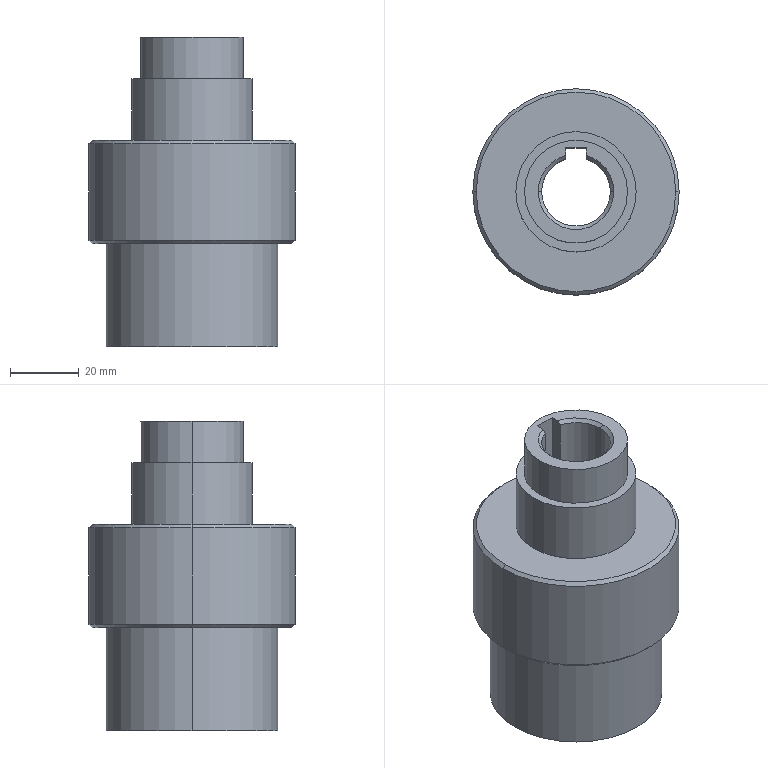Part | SolidWorks | features ICE 8, HoleWzd 2, Chamfer 1, Extrusion 1 | 1 solid | 31 faces | box 60 x 60 x 90 mm | volume 128146 mm3 | cylinder 13 | cone 9 | plane 9 | commonest cylinder face diameters 30 x4 20 x3 35 x2 50 x2 60 x2
STEP:
#1=CARTESIAN_POINT('',(15.,0.,1.));
#2=VERTEX_POINT('',#1);
#3=CARTESIAN_POINT('',(-15.,0.,1.));
#4=VERTEX_POINT('',#3);
#5=CARTESIAN_POINT('',(0.,0.,1.));
#6=DIRECTION('',(0.,0.,-1.));
#7=DIRECTION('',(1.,0.,0.));
#8=AXIS2_PLACEMENT_3D('',#5,#6,#7);
#9=CIRCLE('',#8,15.);
#10=EDGE_CURVE('',#2,#4,#9,.T.);
#11=ORIENTED_EDGE('',*,*,#10,.F.);
#12=CARTESIAN_POINT('',(16.,0.,0.));
#13=VERTEX_POINT('',#12);
#14=CARTESIAN_POINT('',(15.,0.,1.));
#15=DIRECTION('',(0.7071,0.,-0.7071));
#16=VECTOR('',#15,1000.);
#17=LINE('',#14,#16);
#18=EDGE_CURVE('',#2,#13,#17,.T.);
#19=ORIENTED_EDGE('',*,*,#18,.T.);
#20=CARTESIAN_POINT('',(-16.,0.,0.));
#21=VERTEX_POINT('',#20);
#22=CARTESIAN_POINT('',(0.,0.,0.));
#23=DIRECTION('',(0.,0.,1.));
#24=DIRECTION('',(1.,0.,0.));
#25=AXIS2_PLACEMENT_3D('',#22,#23,#24);
#26=CIRCLE('',#25,16.);
#27=EDGE_CURVE('',#21,#13,#26,.T.);
#28=ORIENTED_EDGE('',*,*,#27,.F.);
#29=CARTESIAN_POINT('',(-15.,0.,1.));
#30=DIRECTION('',(-0.7071,0.,-0.7071));
#31=VECTOR('',#30,1000.);
#32=LINE('',#29,#31);
#33=EDGE_CURVE('',#4,#21,#32,.T.);
#34=ORIENTED_EDGE('',*,*,#33,.F.);
#35=EDGE_LOOP('',(#11,#19,#28,#34));
#36=FACE_OUTER_BOUND('',#35,.T.);
#37=CARTESIAN_POINT('',(0.,0.,1.));
#38=DIRECTION('',(0.,0.,-1.));
#39=DIRECTION('',(-1.,0.,0.));
#40=AXIS2_PLACEMENT_3D('',#37,#38,#39);
#41=CONICAL_SURFACE('',#40,15.,0.7854);
#42=ADVANCED_FACE('',(#36),#41,.F.);
#43=CARTESIAN_POINT('',(-10.,0.,89.));
#44=VERTEX_POINT('',#43);
#45=CARTESIAN_POINT('',(10.,0.,89.));
#46=VERTEX_POINT('',#45);
#47=CARTESIAN_POINT('',(0.,0.,89.));
#48=DIRECTION('',(0.,0.,1.));
#49=DIRECTION('',(1.,0.,0.));
#50=AXIS2_PLACEMENT_3D('',#47,#48,#49);
#51=CIRCLE('',#50,10.);
#52=EDGE_CURVE('',#44,#46,#51,.T.);
#53=ORIENTED_EDGE('',*,*,#52,.F.);
#54=CARTESIAN_POINT('',(-11.,0.,90.));
#55=VERTEX_POINT('',#54);
#56=CARTESIAN_POINT('',(-10.,0.,89.));
#57=DIRECTION('',(-0.7071,0.,0.7071));
#58=VECTOR('',#57,1000.);
#59=LINE('',#56,#58);
#60=EDGE_CURVE('',#44,#55,#59,.T.);
#61=ORIENTED_EDGE('',*,*,#60,.T.);
#62=CARTESIAN_POINT('',(11.,0.,90.));
#63=VERTEX_POINT('',#62);
#64=CARTESIAN_POINT('',(0.,0.,90.));
#65=DIRECTION('',(0.,0.,-1.));
#66=DIRECTION('',(1.,0.,0.));
#67=AXIS2_PLACEMENT_3D('',#64,#65,#66);
#68=CIRCLE('',#67,11.);
#69=EDGE_CURVE('',#63,#55,#68,.T.);
#70=ORIENTED_EDGE('',*,*,#69,.F.);
#71=CARTESIAN_POINT('',(10.,0.,89.));
#72=DIRECTION('',(0.7071,0.,0.7071));
#73=VECTOR('',#72,1000.);
#74=LINE('',#71,#73);
#75=EDGE_CURVE('',#46,#63,#74,.T.);
#76=ORIENTED_EDGE('',*,*,#75,.F.);
#77=EDGE_LOOP('',(#53,#61,#70,#76));
#78=FACE_OUTER_BOUND('',#77,.T.);
#79=CARTESIAN_POINT('',(0.,0.,89.));
#80=DIRECTION('',(0.,0.,1.));
#81=DIRECTION('',(1.,0.,0.));
#82=AXIS2_PLACEMENT_3D('',#79,#80,#81);
#83=CONICAL_SURFACE('',#82,10.,0.7854);
#84=ADVANCED_FACE('',(#78),#83,.F.);
#85=CARTESIAN_POINT('',(3.,9.539,89.));
#86=VERTEX_POINT('',#85);
#87=CARTESIAN_POINT('',(0.,0.,89.));
#88=DIRECTION('',(0.,0.,1.));
#89=DIRECTION('',(1.,0.,0.));
#90=AXIS2_PLACEMENT_3D('',#87,#88,#89);
#91=CIRCLE('',#90,10.);
#92=EDGE_CURVE('',#46,#86,#91,.T.);
#93=ORIENTED_EDGE('',*,*,#92,.F.);
#94=ORIENTED_EDGE('',*,*,#75,.T.);
#95=CARTESIAN_POINT('',(3.,10.583,90.));
#96=VERTEX_POINT('',#95);
#97=CARTESIAN_POINT('',(0.,0.,90.));
#98=DIRECTION('',(0.,0.,-1.));
#99=DIRECTION('',(1.,0.,0.));
#100=AXIS2_PLACEMENT_3D('',#97,#98,#99);
#101=CIRCLE('',#100,11.);
#102=EDGE_CURVE('',#96,#63,#101,.T.);
#103=ORIENTED_EDGE('',*,*,#102,.F.);
#104=CARTESIAN_POINT('',(3.,9.539,89.));
#105=CARTESIAN_POINT('',(3.,9.888,89.333));
#106=CARTESIAN_POINT('',(3.,10.236,89.666));
#107=CARTESIAN_POINT('',(3.,10.583,90.));
#108=B_SPLINE_CURVE_WITH_KNOTS('',3,(#104,#105,#106,#107),.UNSPECIFIED.,.F.,.F.,(4,4),(0.,0.001445),.UNSPECIFIED.);
#109=EDGE_CURVE('',#86,#96,#108,.T.);
#110=ORIENTED_EDGE('',*,*,#109,.F.);
#111=EDGE_LOOP('',(#93,#94,#103,#110));
#112=FACE_OUTER_BOUND('',#111,.T.);
#113=CARTESIAN_POINT('',(0.,0.,89.));
#114=DIRECTION('',(0.,0.,1.));
#115=DIRECTION('',(1.,0.,0.));
#116=AXIS2_PLACEMENT_3D('',#113,#114,#115);
#117=CONICAL_SURFACE('',#116,10.,0.7854);
#118=ADVANCED_FACE('',(#112),#117,.F.);
#119=CARTESIAN_POINT('',(-29.,0.,30.));
#120=VERTEX_POINT('',#119);
#121=CARTESIAN_POINT('',(29.,0.,30.));
#122=VERTEX_POINT('',#121);
#123=CARTESIAN_POINT('',(0.,0.,30.));
#124=DIRECTION('',(0.,0.,-1.));
#125=DIRECTION('',(1.,0.,0.));
#126=AXIS2_PLACEMENT_3D('',#123,#124,#125);
#127=CIRCLE('',#126,29.);
#128=EDGE_CURVE('',#120,#122,#127,.T.);
#129=ORIENTED_EDGE('',*,*,#128,.F.);
#130=CARTESIAN_POINT('',(-30.,0.,31.));
#131=VERTEX_POINT('',#130);
#132=CARTESIAN_POINT('',(-30.,0.,31.));
#133=DIRECTION('',(-0.7071,0.,0.7071));
#134=VECTOR('',#133,1000.);
#135=LINE('',#132,#134);
#136=EDGE_CURVE('',#120,#131,#135,.T.);
#137=ORIENTED_EDGE('',*,*,#136,.T.);
#138=CARTESIAN_POINT('',(30.,0.,31.));
#139=VERTEX_POINT('',#138);
#140=CARTESIAN_POINT('',(0.,0.,31.));
#141=DIRECTION('',(0.,0.,1.));
#142=DIRECTION('',(1.,0.,0.));
#143=AXIS2_PLACEMENT_3D('',#140,#141,#142);
#144=CIRCLE('',#143,30.);
#145=EDGE_CURVE('',#139,#131,#144,.T.);
#146=ORIENTED_EDGE('',*,*,#145,.F.);
#147=CARTESIAN_POINT('',(30.,0.,31.));
#148=DIRECTION('',(0.7071,0.,0.7071));
#149=VECTOR('',#148,1000.);
#150=LINE('',#147,#149);
#151=EDGE_CURVE('',#122,#139,#150,.T.);
#152=ORIENTED_EDGE('',*,*,#151,.F.);
#153=EDGE_LOOP('',(#129,#137,#146,#152));
#154=FACE_OUTER_BOUND('',#153,.T.);
#155=CARTESIAN_POINT('',(0.,0.,31.));
#156=DIRECTION('',(0.,0.,1.));
#157=DIRECTION('',(1.,0.,0.));
#158=AXIS2_PLACEMENT_3D('',#155,#156,#157);
#159=CONICAL_SURFACE('',#158,30.,0.7854);
#160=ADVANCED_FACE('',(#154),#159,.T.);
#161=CARTESIAN_POINT('',(29.,0.,60.));
#162=VERTEX_POINT('',#161);
#163=CARTESIAN_POINT('',(-29.,0.,60.));
#164=VERTEX_POINT('',#163);
#165=CARTESIAN_POINT('',(0.,0.,60.));
#166=DIRECTION('',(0.,0.,1.));
#167=DIRECTION('',(1.,0.,0.));
#168=AXIS2_PLACEMENT_3D('',#165,#166,#167);
#169=CIRCLE('',#168,29.);
#170=EDGE_CURVE('',#162,#164,#169,.T.);
#171=ORIENTED_EDGE('',*,*,#170,.F.);
#172=CARTESIAN_POINT('',(30.,0.,59.));
#173=VERTEX_POINT('',#172);
#174=CARTESIAN_POINT('',(29.,0.,60.));
#175=DIRECTION('',(0.7071,0.,-0.7071));
#176=VECTOR('',#175,1000.);
#177=LINE('',#174,#176);
#178=EDGE_CURVE('',#162,#173,#177,.T.);
#179=ORIENTED_EDGE('',*,*,#178,.T.);
#180=CARTESIAN_POINT('',(-30.,0.,59.));
#181=VERTEX_POINT('',#180);
#182=CARTESIAN_POINT('',(0.,0.,59.));
#183=DIRECTION('',(0.,0.,-1.));
#184=DIRECTION('',(1.,0.,0.));
#185=AXIS2_PLACEMENT_3D('',#182,#183,#184);
#186=CIRCLE('',#185,30.);
#187=EDGE_CURVE('',#181,#173,#186,.T.);
#188=ORIENTED_EDGE('',*,*,#187,.F.);
#189=CARTESIAN_POINT('',(-29.,0.,60.));
#190=DIRECTION('',(-0.7071,0.,-0.7071));
#191=VECTOR('',#190,1000.);
#192=LINE('',#189,#191);
#193=EDGE_CURVE('',#164,#181,#192,.T.);
#194=ORIENTED_EDGE('',*,*,#193,.F.);
#195=EDGE_LOOP('',(#171,#179,#188,#194));
#196=FACE_OUTER_BOUND('',#195,.T.);
#197=CARTESIAN_POINT('',(0.,0.,60.));
#198=DIRECTION('',(0.,0.,-1.));
#199=DIRECTION('',(-1.,0.,0.));
#200=AXIS2_PLACEMENT_3D('',#197,#198,#199);
#201=CONICAL_SURFACE('',#200,29.,0.7854);
#202=ADVANCED_FACE('',(#196),#201,.T.);
#203=CARTESIAN_POINT('',(15.,0.,78.));
#204=VERTEX_POINT('',#203);
#205=CARTESIAN_POINT('',(-15.,0.,78.));
#206=VERTEX_POINT('',#205);
#207=CARTESIAN_POINT('',(0.,0.,78.));
#208=DIRECTION('',(0.,0.,1.));
#209=DIRECTION('',(1.,0.,0.));
#210=AXIS2_PLACEMENT_3D('',#207,#208,#209);
#211=CIRCLE('',#210,15.);
#212=EDGE_CURVE('',#204,#206,#211,.T.);
#213=ORIENTED_EDGE('',*,*,#212,.T.);
#214=CARTESIAN_POINT('',(-15.,0.,90.));
#215=VERTEX_POINT('',#214);
#216=CARTESIAN_POINT('',(-15.,0.,78.));
#217=DIRECTION('',(0.,0.,1.));
#218=VECTOR('',#217,1000.);
#219=LINE('',#216,#218);
#220=EDGE_CURVE('',#206,#215,#219,.T.);
#221=ORIENTED_EDGE('',*,*,#220,.T.);
#222=CARTESIAN_POINT('',(15.,0.,90.));
#223=VERTEX_POINT('',#222);
#224=CARTESIAN_POINT('',(0.,0.,90.));
#225=DIRECTION('',(0.,0.,1.));
#226=DIRECTION('',(1.,0.,0.));
#227=AXIS2_PLACEMENT_3D('',#224,#225,#226);
#228=CIRCLE('',#227,15.);
#229=EDGE_CURVE('',#223,#215,#228,.T.);
#230=ORIENTED_EDGE('',*,*,#229,.F.);
#231=CARTESIAN_POINT('',(15.,0.,78.));
#232=DIRECTION('',(0.,0.,1.));
#233=VECTOR('',#232,1000.);
#234=LINE('',#231,#233);
#235=EDGE_CURVE('',#204,#223,#234,.T.);
#236=ORIENTED_EDGE('',*,*,#235,.F.);
#237=EDGE_LOOP('',(#213,#221,#230,#236));
#238=FACE_OUTER_BOUND('',#237,.T.);
#239=CARTESIAN_POINT('',(0.,0.,78.));
#240=DIRECTION('',(0.,0.,1.));
#241=DIRECTION('',(1.,0.,0.));
#242=AXIS2_PLACEMENT_3D('',#239,#240,#241);
#243=CYLINDRICAL_SURFACE('',#242,15.);
#244=ADVANCED_FACE('',(#238),#243,.T.);
#245=CARTESIAN_POINT('',(15.,0.,30.));
#246=VERTEX_POINT('',#245);
#247=CARTESIAN_POINT('',(-15.,0.,30.));
#248=VERTEX_POINT('',#247);
#249=CARTESIAN_POINT('',(0.,0.,30.));
#250=DIRECTION('',(0.,0.,-1.));
#251=DIRECTION('',(-1.,0.,0.));
#252=AXIS2_PLACEMENT_3D('',#249,#250,#251);
#253=CIRCLE('',#252,15.);
#254=EDGE_CURVE('',#246,#248,#253,.T.);
#255=ORIENTED_EDGE('',*,*,#254,.F.);
#256=CARTESIAN_POINT('',(15.,0.,30.));
#257=DIRECTION('',(0.,0.,-1.));
#258=VECTOR('',#257,1000.);
#259=LINE('',#256,#258);
#260=EDGE_CURVE('',#246,#2,#259,.T.);
#261=ORIENTED_EDGE('',*,*,#260,.T.);
#262=ORIENTED_EDGE('',*,*,#10,.T.);
#263=CARTESIAN_POINT('',(-15.,0.,30.));
#264=DIRECTION('',(0.,0.,-1.));
#265=VECTOR('',#264,1000.);
#266=LINE('',#263,#265);
#267=EDGE_CURVE('',#248,#4,#266,.T.);
#268=ORIENTED_EDGE('',*,*,#267,.F.);
#269=EDGE_LOOP('',(#255,#261,#262,#268));
#270=FACE_OUTER_BOUND('',#269,.T.);
#271=CARTESIAN_POINT('',(0.,0.,30.));
#272=DIRECTION('',(0.,0.,-1.));
#273=DIRECTION('',(-1.,0.,0.));
#274=AXIS2_PLACEMENT_3D('',#271,#272,#273);
#275=CYLINDRICAL_SURFACE('',#274,15.);
#276=ADVANCED_FACE('',(#270),#275,.F.);
#277=CARTESIAN_POINT('',(25.,0.,30.));
#278=VERTEX_POINT('',#277);
#279=CARTESIAN_POINT('',(-25.,0.,30.));
#280=VERTEX_POINT('',#279);
#281=CARTESIAN_POINT('',(0.,0.,30.));
#282=DIRECTION('',(0.,0.,1.));
#283=DIRECTION('',(1.,0.,0.));
#284=AXIS2_PLACEMENT_3D('',#281,#282,#283);
#285=CIRCLE('',#284,25.);
#286=EDGE_CURVE('',#278,#280,#285,.T.);
#287=ORIENTED_EDGE('',*,*,#286,.F.);
#288=CARTESIAN_POINT('',(25.,0.,0.));
#289=VERTEX_POINT('',#288);
#290=CARTESIAN_POINT('',(25.,0.,30.));
#291=DIRECTION('',(0.,0.,-1.));
#292=VECTOR('',#291,1000.);
#293=LINE('',#290,#292);
#294=EDGE_CURVE('',#278,#289,#293,.T.);
#295=ORIENTED_EDGE('',*,*,#294,.T.);
#296=CARTESIAN_POINT('',(-25.,0.,0.));
#297=VERTEX_POINT('',#296);
#298=CARTESIAN_POINT('',(0.,0.,0.));
#299=DIRECTION('',(0.,0.,1.));
#300=DIRECTION('',(1.,0.,0.));
#301=AXIS2_PLACEMENT_3D('',#298,#299,#300);
#302=CIRCLE('',#301,25.);
#303=EDGE_CURVE('',#289,#297,#302,.T.);
#304=ORIENTED_EDGE('',*,*,#303,.T.);
#305=CARTESIAN_POINT('',(-25.,0.,30.));
#306=DIRECTION('',(0.,0.,-1.));
#307=VECTOR('',#306,1000.);
#308=LINE('',#305,#307);
#309=EDGE_CURVE('',#280,#297,#308,.T.);
#310=ORIENTED_EDGE('',*,*,#309,.F.);
#311=EDGE_LOOP('',(#287,#295,#304,#310));
#312=FACE_OUTER_BOUND('',#311,.T.);
#313=CARTESIAN_POINT('',(0.,0.,30.));
#314=DIRECTION('',(0.,0.,-1.));
#315=DIRECTION('',(-1.,0.,0.));
#316=AXIS2_PLACEMENT_3D('',#313,#314,#315);
#317=CYLINDRICAL_SURFACE('',#316,25.);
#318=ADVANCED_FACE('',(#312),#317,.T.);
#319=ORIENTED_EDGE('',*,*,#52,.T.);
#320=CARTESIAN_POINT('',(10.,0.,30.));
#321=VERTEX_POINT('',#320);
#322=CARTESIAN_POINT('',(10.,0.,70.));
#323=DIRECTION('',(0.,0.,-1.));
#324=VECTOR('',#323,1000.);
#325=LINE('',#322,#324);
#326=EDGE_CURVE('',#46,#321,#325,.T.);
#327=ORIENTED_EDGE('',*,*,#326,.T.);
#328=CARTESIAN_POINT('',(-10.,0.,30.));
#329=VERTEX_POINT('',#328);
#330=CARTESIAN_POINT('',(0.,0.,30.));
#331=DIRECTION('',(0.,0.,1.));
#332=DIRECTION('',(-1.,0.,0.));
#333=AXIS2_PLACEMENT_3D('',#330,#331,#332);
#334=CIRCLE('',#333,10.);
#335=EDGE_CURVE('',#329,#321,#334,.T.);
#336=ORIENTED_EDGE('',*,*,#335,.F.);
#337=CARTESIAN_POINT('',(-10.,0.,70.));
#338=DIRECTION('',(0.,0.,-1.));
#339=VECTOR('',#338,1000.);
#340=LINE('',#337,#339);
#341=EDGE_CURVE('',#44,#329,#340,.T.);
#342=ORIENTED_EDGE('',*,*,#341,.F.);
#343=EDGE_LOOP('',(#319,#327,#336,#342));
#344=FACE_OUTER_BOUND('',#343,.T.);
#345=CARTESIAN_POINT('',(0.,0.,70.));
#346=DIRECTION('',(0.,0.,-1.));
#347=DIRECTION('',(-1.,0.,0.));
#348=AXIS2_PLACEMENT_3D('',#345,#346,#347);
#349=CYLINDRICAL_SURFACE('',#348,10.);
#350=ADVANCED_FACE('',(#344),#349,.F.);
#351=CARTESIAN_POINT('',(-3.,9.539,89.));
#352=VERTEX_POINT('',#351);
#353=CARTESIAN_POINT('',(0.,0.,89.));
#354=DIRECTION('',(0.,0.,1.));
#355=DIRECTION('',(1.,0.,0.));
#356=AXIS2_PLACEMENT_3D('',#353,#354,#355);
#357=CIRCLE('',#356,10.);
#358=EDGE_CURVE('',#352,#44,#357,.T.);
#359=ORIENTED_EDGE('',*,*,#358,.T.);
#360=ORIENTED_EDGE('',*,*,#341,.T.);
#361=CARTESIAN_POINT('',(-3.,9.539,30.));
#362=VERTEX_POINT('',#361);
#363=CARTESIAN_POINT('',(0.,0.,30.));
#364=DIRECTION('',(0.,0.,1.));
#365=DIRECTION('',(-1.,0.,0.));
#366=AXIS2_PLACEMENT_3D('',#363,#364,#365);
#367=CIRCLE('',#366,10.);
#368=EDGE_CURVE('',#362,#329,#367,.T.);
#369=ORIENTED_EDGE('',*,*,#368,.F.);
#370=CARTESIAN_POINT('',(-3.,9.539,0.));
#371=DIRECTION('',(0.,0.,1.));
#372=VECTOR('',#371,1000.);
#373=LINE('',#370,#372);
#374=EDGE_CURVE('',#362,#352,#373,.T.);
#375=ORIENTED_EDGE('',*,*,#374,.T.);
#376=EDGE_LOOP('',(#359,#360,#369,#375));
#377=FACE_OUTER_BOUND('',#376,.T.);
#378=CARTESIAN_POINT('',(0.,0.,70.));
#379=DIRECTION('',(0.,0.,-1.));
#380=DIRECTION('',(-1.,0.,0.));
#381=AXIS2_PLACEMENT_3D('',#378,#379,#380);
#382=CYLINDRICAL_SURFACE('',#381,10.);
#383=ADVANCED_FACE('',(#377),#382,.F.);
#384=ORIENTED_EDGE('',*,*,#187,.T.);
#385=CARTESIAN_POINT('',(30.,0.,70.));
#386=DIRECTION('',(0.,0.,-1.));
#387=VECTOR('',#386,1000.);
#388=LINE('',#385,#387);
#389=EDGE_CURVE('',#173,#139,#388,.T.);
#390=ORIENTED_EDGE('',*,*,#389,.T.);
#391=ORIENTED_EDGE('',*,*,#145,.T.);
#392=CARTESIAN_POINT('',(-30.,0.,70.));
#393=DIRECTION('',(0.,0.,-1.));
#394=VECTOR('',#393,1000.);
#395=LINE('',#392,#394);
#396=EDGE_CURVE('',#181,#131,#395,.T.);
#397=ORIENTED_EDGE('',*,*,#396,.F.);
#398=EDGE_LOOP('',(#384,#390,#391,#397));
#399=FACE_OUTER_BOUND('',#398,.T.);
#400=CARTESIAN_POINT('',(0.,0.,70.));
#401=DIRECTION('',(0.,0.,-1.));
#402=DIRECTION('',(-1.,0.,0.));
#403=AXIS2_PLACEMENT_3D('',#400,#401,#402);
#404=CYLINDRICAL_SURFACE('',#403,30.);
#405=ADVANCED_FACE('',(#399),#404,.T.);
#406=CARTESIAN_POINT('',(17.5,0.,78.));
#407=VERTEX_POINT('',#406);
#408=CARTESIAN_POINT('',(-17.5,0.,78.));
#409=VERTEX_POINT('',#408);
#410=CARTESIAN_POINT('',(0.,0.,78.));
#411=DIRECTION('',(0.,0.,1.));
#412=DIRECTION('',(1.,0.,0.));
#413=AXIS2_PLACEMENT_3D('',#410,#411,#412);
#414=CIRCLE('',#413,17.5);
#415=EDGE_CURVE('',#407,#409,#414,.T.);
#416=ORIENTED_EDGE('',*,*,#415,.F.);
#417=CARTESIAN_POINT('',(17.5,0.,60.));
#418=VERTEX_POINT('',#417);
#419=CARTESIAN_POINT('',(17.5,0.,90.));
#420=DIRECTION('',(0.,0.,-1.));
#421=VECTOR('',#420,1000.);
#422=LINE('',#419,#421);
#423=EDGE_CURVE('',#407,#418,#422,.T.);
#424=ORIENTED_EDGE('',*,*,#423,.T.);
#425=CARTESIAN_POINT('',(-17.5,0.,60.));
#426=VERTEX_POINT('',#425);
#427=CARTESIAN_POINT('',(0.,0.,60.));
#428=DIRECTION('',(0.,0.,1.));
#429=DIRECTION('',(1.,0.,0.));
#430=AXIS2_PLACEMENT_3D('',#427,#428,#429);
#431=CIRCLE('',#430,17.5);
#432=EDGE_CURVE('',#418,#426,#431,.T.);
#433=ORIENTED_EDGE('',*,*,#432,.T.);
#434=CARTESIAN_POINT('',(-17.5,0.,90.));
#435=DIRECTION('',(0.,0.,-1.));
#436=VECTOR('',#435,1000.);
#437=LINE('',#434,#436);
#438=EDGE_CURVE('',#409,#426,#437,.T.);
#439=ORIENTED_EDGE('',*,*,#438,.F.);
#440=EDGE_LOOP('',(#416,#424,#433,#439));
#441=FACE_OUTER_BOUND('',#440,.T.);
#442=CARTESIAN_POINT('',(0.,0.,90.));
#443=DIRECTION('',(0.,0.,-1.));
#444=DIRECTION('',(-1.,0.,0.));
#445=AXIS2_PLACEMENT_3D('',#442,#443,#444);
#446=CYLINDRICAL_SURFACE('',#445,17.5);
#447=ADVANCED_FACE('',(#441),#446,.T.);
#448=CARTESIAN_POINT('',(3.,12.8,90.));
#449=VERTEX_POINT('',#448);
#450=CARTESIAN_POINT('',(3.,9.539,90.));
#451=DIRECTION('',(0.,1.,0.));
#452=VECTOR('',#451,1000.);
#453=LINE('',#450,#452);
#454=EDGE_CURVE('',#96,#449,#453,.T.);
#455=ORIENTED_EDGE('',*,*,#454,.F.);
#456=ORIENTED_EDGE('',*,*,#102,.T.);
#457=ORIENTED_EDGE('',*,*,#69,.T.);
#458=CARTESIAN_POINT('',(-3.,10.583,90.));
#459=VERTEX_POINT('',#458);
#460=CARTESIAN_POINT('',(0.,0.,90.));
#461=DIRECTION('',(0.,0.,-1.));
#462=DIRECTION('',(1.,0.,0.));
#463=AXIS2_PLACEMENT_3D('',#460,#461,#462);
#464=CIRCLE('',#463,11.);
#465=EDGE_CURVE('',#55,#459,#464,.T.);
#466=ORIENTED_EDGE('',*,*,#465,.T.);
#467=CARTESIAN_POINT('',(-3.,12.8,90.));
#468=VERTEX_POINT('',#467);
#469=CARTESIAN_POINT('',(-3.,12.8,90.));
#470=DIRECTION('',(0.,-1.,0.));
#471=VECTOR('',#470,1000.);
#472=LINE('',#469,#471);
#473=EDGE_CURVE('',#468,#459,#472,.T.);
#474=ORIENTED_EDGE('',*,*,#473,.F.);
#475=CARTESIAN_POINT('',(3.,12.8,90.));
#476=DIRECTION('',(-1.,0.,0.));
#477=VECTOR('',#476,1000.);
#478=LINE('',#475,#477);
#479=EDGE_CURVE('',#449,#468,#478,.T.);
#480=ORIENTED_EDGE('',*,*,#479,.F.);
#481=EDGE_LOOP('',(#455,#456,#457,#466,#474,#480));
#482=FACE_BOUND('',#481,.T.);
#483=ORIENTED_EDGE('',*,*,#229,.T.);
#484=CARTESIAN_POINT('',(0.,0.,90.));
#485=DIRECTION('',(0.,0.,1.));
#486=DIRECTION('',(1.,0.,0.));
#487=AXIS2_PLACEMENT_3D('',#484,#485,#486);
#488=CIRCLE('',#487,15.);
#489=EDGE_CURVE('',#215,#223,#488,.T.);
#490=ORIENTED_EDGE('',*,*,#489,.T.);
#491=EDGE_LOOP('',(#483,#490));
#492=FACE_OUTER_BOUND('',#491,.T.);
#493=CARTESIAN_POINT('',(0.,0.,90.));
#494=DIRECTION('',(0.,0.,1.));
#495=DIRECTION('',(1.,0.,0.));
#496=AXIS2_PLACEMENT_3D('',#493,#494,#495);
#497=PLANE('',#496);
#498=ADVANCED_FACE('',(#482,#492),#497,.T.);
#499=ORIENTED_EDGE('',*,*,#423,.F.);
#500=CARTESIAN_POINT('',(0.,0.,78.));
#501=DIRECTION('',(0.,0.,1.));
#502=DIRECTION('',(1.,0.,0.));
#503=AXIS2_PLACEMENT_3D('',#500,#501,#502);
#504=CIRCLE('',#503,17.5);
#505=EDGE_CURVE('',#409,#407,#504,.T.);
#506=ORIENTED_EDGE('',*,*,#505,.F.);
#507=ORIENTED_EDGE('',*,*,#438,.T.);
#508=CARTESIAN_POINT('',(0.,0.,60.));
#509=DIRECTION('',(0.,0.,1.));
#510=DIRECTION('',(1.,0.,0.));
#511=AXIS2_PLACEMENT_3D('',#508,#509,#510);
#512=CIRCLE('',#511,17.5);
#513=EDGE_CURVE('',#426,#418,#512,.T.);
#514=ORIENTED_EDGE('',*,*,#513,.T.);
#515=EDGE_LOOP('',(#499,#506,#507,#514));
#516=FACE_OUTER_BOUND('',#515,.T.);
#517=CARTESIAN_POINT('',(0.,0.,90.));
#518=DIRECTION('',(0.,0.,-1.));
#519=DIRECTION('',(-1.,0.,0.));
#520=AXIS2_PLACEMENT_3D('',#517,#518,#519);
#521=CYLINDRICAL_SURFACE('',#520,17.5);
#522=ADVANCED_FACE('',(#516),#521,.T.);
#523=ORIENTED_EDGE('',*,*,#389,.F.);
#524=CARTESIAN_POINT('',(0.,0.,59.));
#525=DIRECTION('',(0.,0.,-1.));
#526=DIRECTION('',(1.,0.,0.));
#527=AXIS2_PLACEMENT_3D('',#524,#525,#526);
#528=CIRCLE('',#527,30.);
#529=EDGE_CURVE('',#173,#181,#528,.T.);
#530=ORIENTED_EDGE('',*,*,#529,.T.);
#531=ORIENTED_EDGE('',*,*,#396,.T.);
#532=CARTESIAN_POINT('',(0.,0.,31.));
#533=DIRECTION('',(0.,0.,1.));
#534=DIRECTION('',(1.,0.,0.));
#535=AXIS2_PLACEMENT_3D('',#532,#533,#534);
#536=CIRCLE('',#535,30.);
#537=EDGE_CURVE('',#131,#139,#536,.T.);
#538=ORIENTED_EDGE('',*,*,#537,.T.);
#539=EDGE_LOOP('',(#523,#530,#531,#538));
#540=FACE_OUTER_BOUND('',#539,.T.);
#541=CARTESIAN_POINT('',(0.,0.,70.));
#542=DIRECTION('',(0.,0.,-1.));
#543=DIRECTION('',(-1.,0.,0.));
#544=AXIS2_PLACEMENT_3D('',#541,#542,#543);
#545=CYLINDRICAL_SURFACE('',#544,30.);
#546=ADVANCED_FACE('',(#540),#545,.T.);
#547=ORIENTED_EDGE('',*,*,#326,.F.);
#548=ORIENTED_EDGE('',*,*,#92,.T.);
#549=CARTESIAN_POINT('',(3.,9.539,30.));
#550=VERTEX_POINT('',#549);
#551=CARTESIAN_POINT('',(3.,9.539,0.));
#552=DIRECTION('',(0.,0.,1.));
#553=VECTOR('',#552,1000.);
#554=LINE('',#551,#553);
#555=EDGE_CURVE('',#550,#86,#554,.T.);
#556=ORIENTED_EDGE('',*,*,#555,.F.);
#557=CARTESIAN_POINT('',(0.,0.,30.));
#558=DIRECTION('',(0.,0.,1.));
#559=DIRECTION('',(-1.,0.,0.));
#560=AXIS2_PLACEMENT_3D('',#557,#558,#559);
#561=CIRCLE('',#560,10.);
#562=EDGE_CURVE('',#321,#550,#561,.T.);
#563=ORIENTED_EDGE('',*,*,#562,.F.);
#564=EDGE_LOOP('',(#547,#548,#556,#563));
#565=FACE_OUTER_BOUND('',#564,.T.);
#566=CARTESIAN_POINT('',(0.,0.,70.));
#567=DIRECTION('',(0.,0.,-1.));
#568=DIRECTION('',(-1.,0.,0.));
#569=AXIS2_PLACEMENT_3D('',#566,#567,#568);
#570=CYLINDRICAL_SURFACE('',#569,10.);
#571=ADVANCED_FACE('',(#565),#570,.F.);
#572=ORIENTED_EDGE('',*,*,#555,.T.);
#573=ORIENTED_EDGE('',*,*,#109,.T.);
#574=ORIENTED_EDGE('',*,*,#454,.T.);
#575=CARTESIAN_POINT('',(3.,12.8,30.));
#576=VERTEX_POINT('',#575);
#577=CARTESIAN_POINT('',(3.,12.8,0.));
#578=DIRECTION('',(0.,0.,1.));
#579=VECTOR('',#578,1000.);
#580=LINE('',#577,#579);
#581=EDGE_CURVE('',#576,#449,#580,.T.);
#582=ORIENTED_EDGE('',*,*,#581,.F.);
#583=CARTESIAN_POINT('',(3.,9.539,30.));
#584=DIRECTION('',(0.,1.,0.));
#585=VECTOR('',#584,1000.);
#586=LINE('',#583,#585);
#587=EDGE_CURVE('',#550,#576,#586,.T.);
#588=ORIENTED_EDGE('',*,*,#587,.F.);
#589=EDGE_LOOP('',(#572,#573,#574,#582,#588));
#590=FACE_OUTER_BOUND('',#589,.T.);
#591=CARTESIAN_POINT('',(3.,9.539,0.));
#592=DIRECTION('',(1.,0.,0.));
#593=DIRECTION('',(0.,0.,-1.));
#594=AXIS2_PLACEMENT_3D('',#591,#592,#593);
#595=PLANE('',#594);
#596=ADVANCED_FACE('',(#590),#595,.F.);
#597=ORIENTED_EDGE('',*,*,#473,.T.);
#598=CARTESIAN_POINT('',(-3.,10.583,90.));
#599=CARTESIAN_POINT('',(-3.,10.236,89.666));
#600=CARTESIAN_POINT('',(-3.,9.888,89.333));
#601=CARTESIAN_POINT('',(-3.,9.539,89.));
#602=B_SPLINE_CURVE_WITH_KNOTS('',3,(#598,#599,#600,#601),.UNSPECIFIED.,.F.,.F.,(4,4),(0.,0.001445),.UNSPECIFIED.);
#603=EDGE_CURVE('',#459,#352,#602,.T.);
#604=ORIENTED_EDGE('',*,*,#603,.T.);
#605=ORIENTED_EDGE('',*,*,#374,.F.);
#606=CARTESIAN_POINT('',(-3.,12.8,30.));
#607=VERTEX_POINT('',#606);
#608=CARTESIAN_POINT('',(-3.,9.539,30.));
#609=DIRECTION('',(0.,-1.,0.));
#610=VECTOR('',#609,1000.);
#611=LINE('',#608,#610);
#612=EDGE_CURVE('',#607,#362,#611,.T.);
#613=ORIENTED_EDGE('',*,*,#612,.F.);
#614=CARTESIAN_POINT('',(-3.,12.8,0.));
#615=DIRECTION('',(0.,0.,1.));
#616=VECTOR('',#615,1000.);
#617=LINE('',#614,#616);
#618=EDGE_CURVE('',#607,#468,#617,.T.);
#619=ORIENTED_EDGE('',*,*,#618,.T.);
#620=EDGE_LOOP('',(#597,#604,#605,#613,#619));
#621=FACE_OUTER_BOUND('',#620,.T.);
#622=CARTESIAN_POINT('',(-3.,9.539,0.));
#623=DIRECTION('',(-1.,0.,0.));
#624=DIRECTION('',(0.,0.,1.));
#625=AXIS2_PLACEMENT_3D('',#622,#623,#624);
#626=PLANE('',#625);
#627=ADVANCED_FACE('',(#621),#626,.F.);
#628=CARTESIAN_POINT('',(-3.,12.8,30.));
#629=DIRECTION('',(-1.,0.,0.));
#630=VECTOR('',#629,1000.);
#631=LINE('',#628,#630);
#632=EDGE_CURVE('',#576,#607,#631,.T.);
#633=ORIENTED_EDGE('',*,*,#632,.F.);
#634=ORIENTED_EDGE('',*,*,#581,.T.);
#635=ORIENTED_EDGE('',*,*,#479,.T.);
#636=ORIENTED_EDGE('',*,*,#618,.F.);
#637=EDGE_LOOP('',(#633,#634,#635,#636));
#638=FACE_OUTER_BOUND('',#637,.T.);
#639=CARTESIAN_POINT('',(-3.,12.8,0.));
#640=DIRECTION('',(0.,1.,0.));
#641=DIRECTION('',(0.,0.,1.));
#642=AXIS2_PLACEMENT_3D('',#639,#640,#641);
#643=PLANE('',#642);
#644=ADVANCED_FACE('',(#638),#643,.F.);
#645=ORIENTED_EDGE('',*,*,#294,.F.);
#646=CARTESIAN_POINT('',(0.,0.,30.));
#647=DIRECTION('',(0.,0.,1.));
#648=DIRECTION('',(1.,0.,0.));
#649=AXIS2_PLACEMENT_3D('',#646,#647,#648);
#650=CIRCLE('',#649,25.);
#651=EDGE_CURVE('',#280,#278,#650,.T.);
#652=ORIENTED_EDGE('',*,*,#651,.F.);
#653=ORIENTED_EDGE('',*,*,#309,.T.);
#654=CARTESIAN_POINT('',(0.,0.,0.));
#655=DIRECTION('',(0.,0.,1.));
#656=DIRECTION('',(1.,0.,0.));
#657=AXIS2_PLACEMENT_3D('',#654,#655,#656);
#658=CIRCLE('',#657,25.);
#659=EDGE_CURVE('',#297,#289,#658,.T.);
#660=ORIENTED_EDGE('',*,*,#659,.T.);
#661=EDGE_LOOP('',(#645,#652,#653,#660));
#662=FACE_OUTER_BOUND('',#661,.T.);
#663=CARTESIAN_POINT('',(0.,0.,30.));
#664=DIRECTION('',(0.,0.,-1.));
#665=DIRECTION('',(-1.,0.,0.));
#666=AXIS2_PLACEMENT_3D('',#663,#664,#665);
#667=CYLINDRICAL_SURFACE('',#666,25.);
#668=ADVANCED_FACE('',(#662),#667,.T.);
#669=ORIENTED_EDGE('',*,*,#27,.T.);
#670=CARTESIAN_POINT('',(0.,0.,0.));
#671=DIRECTION('',(0.,0.,1.));
#672=DIRECTION('',(1.,0.,0.));
#673=AXIS2_PLACEMENT_3D('',#670,#671,#672);
#674=CIRCLE('',#673,16.);
#675=EDGE_CURVE('',#13,#21,#674,.T.);
#676=ORIENTED_EDGE('',*,*,#675,.T.);
#677=EDGE_LOOP('',(#669,#676));
#678=FACE_BOUND('',#677,.T.);
#679=ORIENTED_EDGE('',*,*,#659,.F.);
#680=ORIENTED_EDGE('',*,*,#303,.F.);
#681=EDGE_LOOP('',(#679,#680));
#682=FACE_OUTER_BOUND('',#681,.T.);
#683=CARTESIAN_POINT('',(0.,0.,0.));
#684=DIRECTION('',(0.,0.,1.));
#685=DIRECTION('',(1.,0.,0.));
#686=AXIS2_PLACEMENT_3D('',#683,#684,#685);
#687=PLANE('',#686);
#688=ADVANCED_FACE('',(#678,#682),#687,.F.);
#689=CARTESIAN_POINT('',(0.,0.,30.));
#690=DIRECTION('',(0.,0.,-1.));
#691=DIRECTION('',(1.,0.,0.));
#692=AXIS2_PLACEMENT_3D('',#689,#690,#691);
#693=CIRCLE('',#692,29.);
#694=EDGE_CURVE('',#122,#120,#693,.T.);
#695=ORIENTED_EDGE('',*,*,#694,.T.);
#696=ORIENTED_EDGE('',*,*,#128,.T.);
#697=EDGE_LOOP('',(#695,#696));
#698=FACE_OUTER_BOUND('',#697,.T.);
#699=ORIENTED_EDGE('',*,*,#651,.T.);
#700=ORIENTED_EDGE('',*,*,#286,.T.);
#701=EDGE_LOOP('',(#699,#700));
#702=FACE_BOUND('',#701,.T.);
#703=CARTESIAN_POINT('',(0.,0.,30.));
#704=DIRECTION('',(0.,0.,1.));
#705=DIRECTION('',(1.,0.,0.));
#706=AXIS2_PLACEMENT_3D('',#703,#704,#705);
#707=PLANE('',#706);
#708=ADVANCED_FACE('',(#698,#702),#707,.F.);
#709=CARTESIAN_POINT('',(0.,0.,30.));
#710=DIRECTION('',(0.,0.,-1.));
#711=DIRECTION('',(-1.,0.,0.));
#712=AXIS2_PLACEMENT_3D('',#709,#710,#711);
#713=CIRCLE('',#712,15.);
#714=EDGE_CURVE('',#248,#246,#713,.T.);
#715=ORIENTED_EDGE('',*,*,#714,.T.);
#716=ORIENTED_EDGE('',*,*,#254,.T.);
#717=EDGE_LOOP('',(#715,#716));
#718=FACE_OUTER_BOUND('',#717,.T.);
#719=ORIENTED_EDGE('',*,*,#368,.T.);
#720=ORIENTED_EDGE('',*,*,#335,.T.);
#721=ORIENTED_EDGE('',*,*,#562,.T.);
#722=ORIENTED_EDGE('',*,*,#587,.T.);
#723=ORIENTED_EDGE('',*,*,#632,.T.);
#724=ORIENTED_EDGE('',*,*,#612,.T.);
#725=EDGE_LOOP('',(#719,#720,#721,#722,#723,#724));
#726=FACE_BOUND('',#725,.T.);
#727=CARTESIAN_POINT('',(0.,0.,30.));
#728=DIRECTION('',(0.,0.,-1.));
#729=DIRECTION('',(-1.,0.,0.));
#730=AXIS2_PLACEMENT_3D('',#727,#728,#729);
#731=PLANE('',#730);
#732=ADVANCED_FACE('',(#718,#726),#731,.T.);
#733=ORIENTED_EDGE('',*,*,#260,.F.);
#734=ORIENTED_EDGE('',*,*,#714,.F.);
#735=ORIENTED_EDGE('',*,*,#267,.T.);
#736=CARTESIAN_POINT('',(0.,0.,1.));
#737=DIRECTION('',(0.,0.,-1.));
#738=DIRECTION('',(1.,0.,0.));
#739=AXIS2_PLACEMENT_3D('',#736,#737,#738);
#740=CIRCLE('',#739,15.);
#741=EDGE_CURVE('',#4,#2,#740,.T.);
#742=ORIENTED_EDGE('',*,*,#741,.T.);
#743=EDGE_LOOP('',(#733,#734,#735,#742));
#744=FACE_OUTER_BOUND('',#743,.T.);
#745=CARTESIAN_POINT('',(0.,0.,30.));
#746=DIRECTION('',(0.,0.,-1.));
#747=DIRECTION('',(-1.,0.,0.));
#748=AXIS2_PLACEMENT_3D('',#745,#746,#747);
#749=CYLINDRICAL_SURFACE('',#748,15.);
#750=ADVANCED_FACE('',(#744),#749,.F.);
#751=CARTESIAN_POINT('',(0.,0.,60.));
#752=DIRECTION('',(0.,0.,1.));
#753=DIRECTION('',(1.,0.,0.));
#754=AXIS2_PLACEMENT_3D('',#751,#752,#753);
#755=CIRCLE('',#754,29.);
#756=EDGE_CURVE('',#164,#162,#755,.T.);
#757=ORIENTED_EDGE('',*,*,#756,.T.);
#758=ORIENTED_EDGE('',*,*,#170,.T.);
#759=EDGE_LOOP('',(#757,#758));
#760=FACE_OUTER_BOUND('',#759,.T.);
#761=ORIENTED_EDGE('',*,*,#513,.F.);
#762=ORIENTED_EDGE('',*,*,#432,.F.);
#763=EDGE_LOOP('',(#761,#762));
#764=FACE_BOUND('',#763,.T.);
#765=CARTESIAN_POINT('',(0.,0.,60.));
#766=DIRECTION('',(0.,0.,1.));
#767=DIRECTION('',(1.,0.,0.));
#768=AXIS2_PLACEMENT_3D('',#765,#766,#767);
#769=PLANE('',#768);
#770=ADVANCED_FACE('',(#760,#764),#769,.T.);
#771=ORIENTED_EDGE('',*,*,#212,.F.);
#772=CARTESIAN_POINT('',(0.,0.,78.));
#773=DIRECTION('',(0.,0.,1.));
#774=DIRECTION('',(1.,0.,0.));
#775=AXIS2_PLACEMENT_3D('',#772,#773,#774);
#776=CIRCLE('',#775,15.);
#777=EDGE_CURVE('',#206,#204,#776,.T.);
#778=ORIENTED_EDGE('',*,*,#777,.F.);
#779=EDGE_LOOP('',(#771,#778));
#780=FACE_BOUND('',#779,.T.);
#781=ORIENTED_EDGE('',*,*,#505,.T.);
#782=ORIENTED_EDGE('',*,*,#415,.T.);
#783=EDGE_LOOP('',(#781,#782));
#784=FACE_OUTER_BOUND('',#783,.T.);
#785=CARTESIAN_POINT('',(0.,0.,78.));
#786=DIRECTION('',(0.,0.,1.));
#787=DIRECTION('',(1.,0.,0.));
#788=AXIS2_PLACEMENT_3D('',#785,#786,#787);
#789=PLANE('',#788);
#790=ADVANCED_FACE('',(#780,#784),#789,.T.);
#791=ORIENTED_EDGE('',*,*,#220,.F.);
#792=ORIENTED_EDGE('',*,*,#777,.T.);
#793=ORIENTED_EDGE('',*,*,#235,.T.);
#794=ORIENTED_EDGE('',*,*,#489,.F.);
#795=EDGE_LOOP('',(#791,#792,#793,#794));
#796=FACE_OUTER_BOUND('',#795,.T.);
#797=CARTESIAN_POINT('',(0.,0.,78.));
#798=DIRECTION('',(0.,0.,1.));
#799=DIRECTION('',(1.,0.,0.));
#800=AXIS2_PLACEMENT_3D('',#797,#798,#799);
#801=CYLINDRICAL_SURFACE('',#800,15.);
#802=ADVANCED_FACE('',(#796),#801,.T.);
#803=ORIENTED_EDGE('',*,*,#178,.F.);
#804=ORIENTED_EDGE('',*,*,#756,.F.);
#805=ORIENTED_EDGE('',*,*,#193,.T.);
#806=ORIENTED_EDGE('',*,*,#529,.F.);
#807=EDGE_LOOP('',(#803,#804,#805,#806));
#808=FACE_OUTER_BOUND('',#807,.T.);
#809=CARTESIAN_POINT('',(0.,0.,60.));
#810=DIRECTION('',(0.,0.,-1.));
#811=DIRECTION('',(-1.,0.,0.));
#812=AXIS2_PLACEMENT_3D('',#809,#810,#811);
#813=CONICAL_SURFACE('',#812,29.,0.7854);
#814=ADVANCED_FACE('',(#808),#813,.T.);
#815=ORIENTED_EDGE('',*,*,#136,.F.);
#816=ORIENTED_EDGE('',*,*,#694,.F.);
#817=ORIENTED_EDGE('',*,*,#151,.T.);
#818=ORIENTED_EDGE('',*,*,#537,.F.);
#819=EDGE_LOOP('',(#815,#816,#817,#818));
#820=FACE_OUTER_BOUND('',#819,.T.);
#821=CARTESIAN_POINT('',(0.,0.,31.));
#822=DIRECTION('',(0.,0.,1.));
#823=DIRECTION('',(1.,0.,0.));
#824=AXIS2_PLACEMENT_3D('',#821,#822,#823);
#825=CONICAL_SURFACE('',#824,30.,0.7854);
#826=ADVANCED_FACE('',(#820),#825,.T.);
#827=ORIENTED_EDGE('',*,*,#60,.F.);
#828=ORIENTED_EDGE('',*,*,#358,.F.);
#829=ORIENTED_EDGE('',*,*,#603,.F.);
#830=ORIENTED_EDGE('',*,*,#465,.F.);
#831=EDGE_LOOP('',(#827,#828,#829,#830));
#832=FACE_OUTER_BOUND('',#831,.T.);
#833=CARTESIAN_POINT('',(0.,0.,89.));
#834=DIRECTION('',(0.,0.,1.));
#835=DIRECTION('',(1.,0.,0.));
#836=AXIS2_PLACEMENT_3D('',#833,#834,#835);
#837=CONICAL_SURFACE('',#836,10.,0.7854);
#838=ADVANCED_FACE('',(#832),#837,.F.);
#839=ORIENTED_EDGE('',*,*,#18,.F.);
#840=ORIENTED_EDGE('',*,*,#741,.F.);
#841=ORIENTED_EDGE('',*,*,#33,.T.);
#842=ORIENTED_EDGE('',*,*,#675,.F.);
#843=EDGE_LOOP('',(#839,#840,#841,#842));
#844=FACE_OUTER_BOUND('',#843,.T.);
#845=CARTESIAN_POINT('',(0.,0.,1.));
#846=DIRECTION('',(0.,0.,-1.));
#847=DIRECTION('',(-1.,0.,0.));
#848=AXIS2_PLACEMENT_3D('',#845,#846,#847);
#849=CONICAL_SURFACE('',#848,15.,0.7854);
#850=ADVANCED_FACE('',(#844),#849,.F.);
#851=CLOSED_SHELL('',(#42,#84,#118,#160,#202,#244,#276,#318,#350,#383,#405,#447,#498,#522,#546,#571,#596,#627,#644,#668,#688,#708,#732,#750,#770,#790,#802,#814,#826,#838,#850));
#852=MANIFOLD_SOLID_BREP('',#851);
#853=CARTESIAN_POINT('',(0.,0.,0.));
#854=DIRECTION('',(0.,0.,1.));
#855=DIRECTION('',(1.,0.,0.));
#856=AXIS2_PLACEMENT_3D('',#853,#854,#855);
#857=(LENGTH_UNIT()NAMED_UNIT(*)SI_UNIT(.MILLI.,.METRE.));
#858=UNCERTAINTY_MEASURE_WITH_UNIT(LENGTH_MEASURE(0.00001),#857,'','');
#859=(NAMED_UNIT(*)PLANE_ANGLE_UNIT()SI_UNIT($,.RADIAN.));
#860=(NAMED_UNIT(*)SI_UNIT($,.STERADIAN.)SOLID_ANGLE_UNIT());
#861=(GEOMETRIC_REPRESENTATION_CONTEXT(3)GLOBAL_UNCERTAINTY_ASSIGNED_CONTEXT((#858))GLOBAL_UNIT_ASSIGNED_CONTEXT((#857,#859,#860))REPRESENTATION_CONTEXT('',''));
#862=ADVANCED_BREP_SHAPE_REPRESENTATION('',(#852,#856),#861);